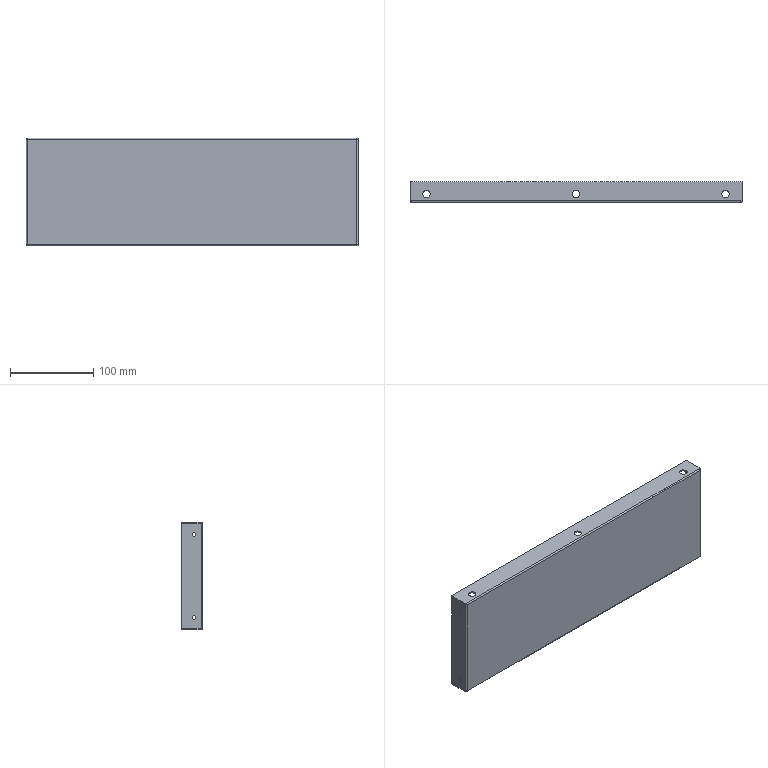Part | STEP file | belt support plate | 1 solid | 62 faces | box 400 x 25 x 130 mm | volume 113936 mm3 | plane 34 | cylinder 28 | commonest cylinder face diameters 9 x12 4.2 x8 0.1 x4 3.1 x4